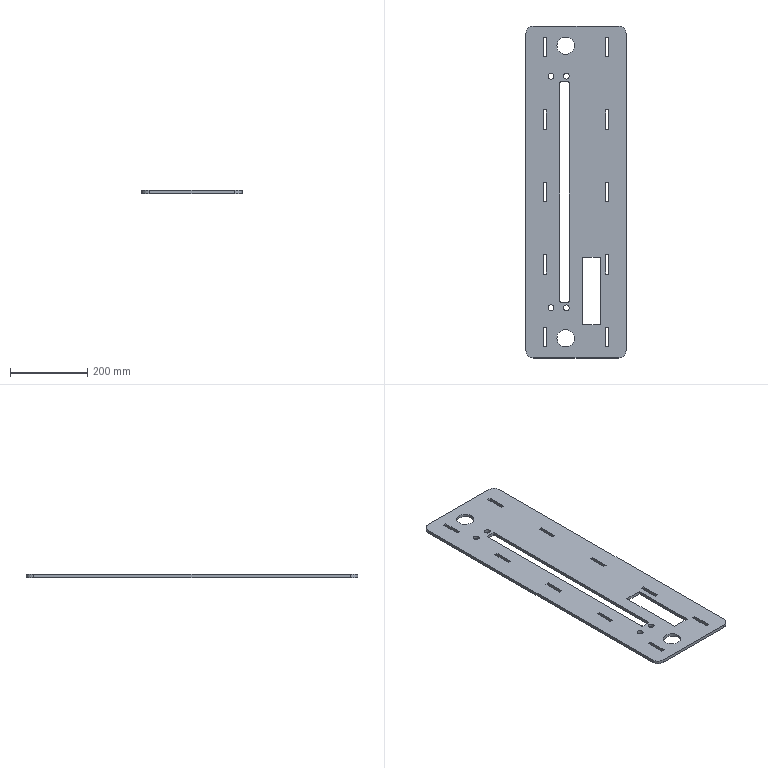Part | SolidWorks | features FlatPattern 1, SMBaseFlange 1, SheetMetal 1 | 1 solid | 74 faces | box 260 x 860 x 8 mm | volume 1544579 mm3 | plane 54 | cylinder 20 | commonest cylinder face diameters 15 x8 4 x4 40 x4 45 x4